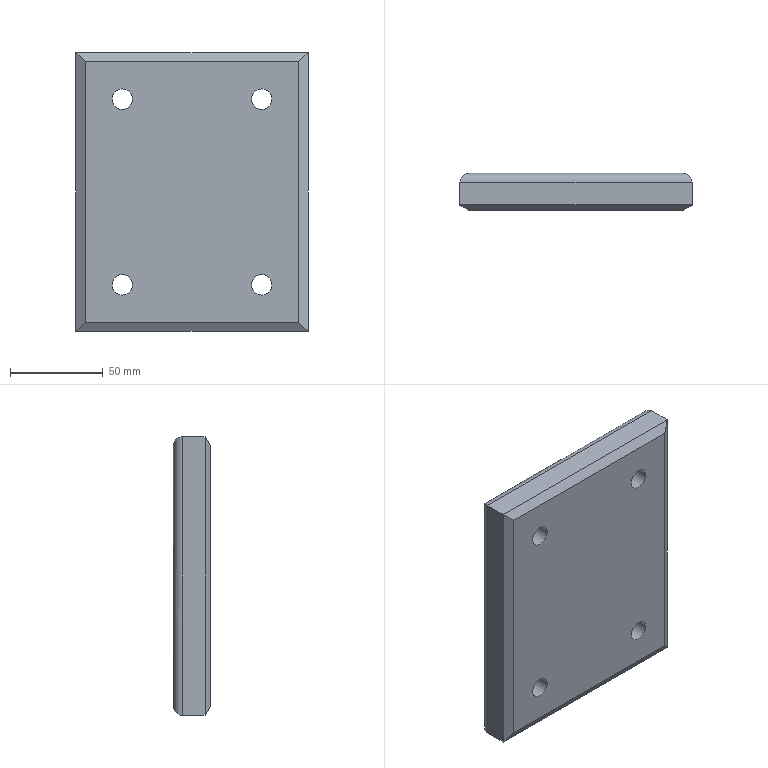Part | NX | features solid 2 | 1 solid | 30 faces | box 125 x 20 x 150 mm | volume 353028 mm3 | plane 14 | cylinder 12 | torus 4 | commonest cylinder face diameters 10 x4 11 x4 17.5 x4
STEP:
#1=CARTESIAN_POINT('',(525.,95.,-285.));
#2=VERTEX_POINT('',#1);
#3=CARTESIAN_POINT('',(640.,95.,-285.));
#4=VERTEX_POINT('',#3);
#5=CARTESIAN_POINT('',(495.,95.,-285.));
#6=DIRECTION('',(1.,0.,0.));
#7=VECTOR('',#6,1000.);
#8=LINE('',#5,#7);
#9=EDGE_CURVE('',#2,#4,#8,.T.);
#10=ORIENTED_EDGE('',*,*,#9,.F.);
#11=CARTESIAN_POINT('',(525.,95.,-145.));
#12=VERTEX_POINT('',#11);
#13=CARTESIAN_POINT('',(525.,95.,-290.));
#14=DIRECTION('',(0.,0.,-1.));
#15=VECTOR('',#14,1000.);
#16=LINE('',#13,#15);
#17=EDGE_CURVE('',#12,#2,#16,.T.);
#18=ORIENTED_EDGE('',*,*,#17,.F.);
#19=CARTESIAN_POINT('',(640.,95.,-145.));
#20=VERTEX_POINT('',#19);
#21=CARTESIAN_POINT('',(495.,95.,-145.));
#22=DIRECTION('',(-1.,0.,0.));
#23=VECTOR('',#22,1000.);
#24=LINE('',#21,#23);
#25=EDGE_CURVE('',#20,#12,#24,.T.);
#26=ORIENTED_EDGE('',*,*,#25,.F.);
#27=CARTESIAN_POINT('',(640.,95.,-290.));
#28=DIRECTION('',(0.,0.,1.));
#29=VECTOR('',#28,1000.);
#30=LINE('',#27,#29);
#31=EDGE_CURVE('',#4,#20,#30,.T.);
#32=ORIENTED_EDGE('',*,*,#31,.F.);
#33=EDGE_LOOP('',(#10,#18,#26,#32));
#34=FACE_BOUND('',#33,.T.);
#35=CARTESIAN_POINT('',(545.,95.,-253.25));
#36=VERTEX_POINT('',#35);
#37=CARTESIAN_POINT('',(545.,95.,-265.));
#38=DIRECTION('',(0.,1.,0.));
#39=DIRECTION('',(0.,0.,1.));
#40=AXIS2_PLACEMENT_3D('',#37,#38,#39);
#41=CIRCLE('',#40,11.75);
#42=EDGE_CURVE('',#36,#36,#41,.T.);
#43=ORIENTED_EDGE('',*,*,#42,.F.);
#44=EDGE_LOOP('',(#43));
#45=FACE_BOUND('',#44,.T.);
#46=CARTESIAN_POINT('',(620.,95.,-253.25));
#47=VERTEX_POINT('',#46);
#48=CARTESIAN_POINT('',(620.,95.,-265.));
#49=DIRECTION('',(0.,1.,0.));
#50=DIRECTION('',(0.,0.,1.));
#51=AXIS2_PLACEMENT_3D('',#48,#49,#50);
#52=CIRCLE('',#51,11.75);
#53=EDGE_CURVE('',#47,#47,#52,.T.);
#54=ORIENTED_EDGE('',*,*,#53,.F.);
#55=EDGE_LOOP('',(#54));
#56=FACE_BOUND('',#55,.T.);
#57=CARTESIAN_POINT('',(620.,95.,-153.25));
#58=VERTEX_POINT('',#57);
#59=CARTESIAN_POINT('',(620.,95.,-165.));
#60=DIRECTION('',(0.,1.,0.));
#61=DIRECTION('',(0.,0.,1.));
#62=AXIS2_PLACEMENT_3D('',#59,#60,#61);
#63=CIRCLE('',#62,11.75);
#64=EDGE_CURVE('',#58,#58,#63,.T.);
#65=ORIENTED_EDGE('',*,*,#64,.F.);
#66=EDGE_LOOP('',(#65));
#67=FACE_BOUND('',#66,.T.);
#68=CARTESIAN_POINT('',(545.,95.,-153.25));
#69=VERTEX_POINT('',#68);
#70=CARTESIAN_POINT('',(545.,95.,-165.));
#71=DIRECTION('',(0.,1.,0.));
#72=DIRECTION('',(0.,0.,1.));
#73=AXIS2_PLACEMENT_3D('',#70,#71,#72);
#74=CIRCLE('',#73,11.75);
#75=EDGE_CURVE('',#69,#69,#74,.T.);
#76=ORIENTED_EDGE('',*,*,#75,.F.);
#77=EDGE_LOOP('',(#76));
#78=FACE_BOUND('',#77,.T.);
#79=CARTESIAN_POINT('',(495.,95.,-290.));
#80=DIRECTION('',(0.,1.,0.));
#81=DIRECTION('',(0.,0.,-1.));
#82=AXIS2_PLACEMENT_3D('',#79,#80,#81);
#83=PLANE('',#82);
#84=ADVANCED_FACE('',(#34,#45,#56,#67,#78),#83,.T.);
#85=CARTESIAN_POINT('',(645.,90.,-140.));
#86=VERTEX_POINT('',#85);
#87=CARTESIAN_POINT('',(645.,78.,-140.));
#88=VERTEX_POINT('',#87);
#89=CARTESIAN_POINT('',(645.,95.,-140.));
#90=DIRECTION('',(0.,-1.,0.));
#91=VECTOR('',#90,1000.);
#92=LINE('',#89,#91);
#93=EDGE_CURVE('',#86,#88,#92,.T.);
#94=ORIENTED_EDGE('',*,*,#93,.F.);
#95=CARTESIAN_POINT('',(520.,90.,-140.));
#96=VERTEX_POINT('',#95);
#97=CARTESIAN_POINT('',(495.,90.,-140.));
#98=DIRECTION('',(1.,0.,0.));
#99=VECTOR('',#98,1000.);
#100=LINE('',#97,#99);
#101=EDGE_CURVE('',#96,#86,#100,.T.);
#102=ORIENTED_EDGE('',*,*,#101,.F.);
#103=CARTESIAN_POINT('',(520.,78.,-140.));
#104=VERTEX_POINT('',#103);
#105=CARTESIAN_POINT('',(520.,95.,-140.));
#106=DIRECTION('',(0.,-1.,0.));
#107=VECTOR('',#106,1000.);
#108=LINE('',#105,#107);
#109=EDGE_CURVE('',#96,#104,#108,.T.);
#110=ORIENTED_EDGE('',*,*,#109,.T.);
#111=CARTESIAN_POINT('',(495.,78.,-140.));
#112=DIRECTION('',(-1.,0.,0.));
#113=VECTOR('',#112,1000.);
#114=LINE('',#111,#113);
#115=EDGE_CURVE('',#88,#104,#114,.T.);
#116=ORIENTED_EDGE('',*,*,#115,.F.);
#117=EDGE_LOOP('',(#94,#102,#110,#116));
#118=FACE_BOUND('',#117,.T.);
#119=CARTESIAN_POINT('',(495.,95.,-140.));
#120=DIRECTION('',(0.,0.,1.));
#121=DIRECTION('',(0.,1.,0.));
#122=AXIS2_PLACEMENT_3D('',#119,#120,#121);
#123=PLANE('',#122);
#124=ADVANCED_FACE('',(#118),#123,.T.);
#125=CARTESIAN_POINT('',(640.,75.,-145.));
#126=VERTEX_POINT('',#125);
#127=CARTESIAN_POINT('',(640.,75.,-285.));
#128=VERTEX_POINT('',#127);
#129=CARTESIAN_POINT('',(640.,75.,-290.));
#130=DIRECTION('',(0.,0.,-1.));
#131=VECTOR('',#130,1000.);
#132=LINE('',#129,#131);
#133=EDGE_CURVE('',#126,#128,#132,.T.);
#134=ORIENTED_EDGE('',*,*,#133,.F.);
#135=CARTESIAN_POINT('',(525.,75.,-145.));
#136=VERTEX_POINT('',#135);
#137=CARTESIAN_POINT('',(495.,75.,-145.));
#138=DIRECTION('',(1.,0.,0.));
#139=VECTOR('',#138,1000.);
#140=LINE('',#137,#139);
#141=EDGE_CURVE('',#136,#126,#140,.T.);
#142=ORIENTED_EDGE('',*,*,#141,.F.);
#143=CARTESIAN_POINT('',(525.,75.,-285.));
#144=VERTEX_POINT('',#143);
#145=CARTESIAN_POINT('',(525.,75.,-140.));
#146=DIRECTION('',(0.,0.,1.));
#147=VECTOR('',#146,1000.);
#148=LINE('',#145,#147);
#149=EDGE_CURVE('',#144,#136,#148,.T.);
#150=ORIENTED_EDGE('',*,*,#149,.F.);
#151=CARTESIAN_POINT('',(495.,75.,-285.));
#152=DIRECTION('',(-1.,0.,0.));
#153=VECTOR('',#152,1000.);
#154=LINE('',#151,#153);
#155=EDGE_CURVE('',#128,#144,#154,.T.);
#156=ORIENTED_EDGE('',*,*,#155,.F.);
#157=EDGE_LOOP('',(#134,#142,#150,#156));
#158=FACE_BOUND('',#157,.T.);
#159=CARTESIAN_POINT('',(620.,75.,-259.5));
#160=VERTEX_POINT('',#159);
#161=CARTESIAN_POINT('',(620.,75.,-265.));
#162=DIRECTION('',(0.,1.,0.));
#163=DIRECTION('',(0.,0.,1.));
#164=AXIS2_PLACEMENT_3D('',#161,#162,#163);
#165=CIRCLE('',#164,5.5);
#166=EDGE_CURVE('',#160,#160,#165,.T.);
#167=ORIENTED_EDGE('',*,*,#166,.T.);
#168=EDGE_LOOP('',(#167));
#169=FACE_BOUND('',#168,.T.);
#170=CARTESIAN_POINT('',(545.,75.,-259.5));
#171=VERTEX_POINT('',#170);
#172=CARTESIAN_POINT('',(545.,75.,-265.));
#173=DIRECTION('',(0.,1.,0.));
#174=DIRECTION('',(0.,0.,1.));
#175=AXIS2_PLACEMENT_3D('',#172,#173,#174);
#176=CIRCLE('',#175,5.5);
#177=EDGE_CURVE('',#171,#171,#176,.T.);
#178=ORIENTED_EDGE('',*,*,#177,.T.);
#179=EDGE_LOOP('',(#178));
#180=FACE_BOUND('',#179,.T.);
#181=CARTESIAN_POINT('',(620.,75.,-159.5));
#182=VERTEX_POINT('',#181);
#183=CARTESIAN_POINT('',(620.,75.,-165.));
#184=DIRECTION('',(0.,1.,0.));
#185=DIRECTION('',(0.,0.,1.));
#186=AXIS2_PLACEMENT_3D('',#183,#184,#185);
#187=CIRCLE('',#186,5.5);
#188=EDGE_CURVE('',#182,#182,#187,.T.);
#189=ORIENTED_EDGE('',*,*,#188,.T.);
#190=EDGE_LOOP('',(#189));
#191=FACE_BOUND('',#190,.T.);
#192=CARTESIAN_POINT('',(545.,75.,-159.5));
#193=VERTEX_POINT('',#192);
#194=CARTESIAN_POINT('',(545.,75.,-165.));
#195=DIRECTION('',(0.,1.,0.));
#196=DIRECTION('',(0.,0.,1.));
#197=AXIS2_PLACEMENT_3D('',#194,#195,#196);
#198=CIRCLE('',#197,5.5);
#199=EDGE_CURVE('',#193,#193,#198,.T.);
#200=ORIENTED_EDGE('',*,*,#199,.T.);
#201=EDGE_LOOP('',(#200));
#202=FACE_BOUND('',#201,.T.);
#203=CARTESIAN_POINT('',(495.,75.,-290.));
#204=DIRECTION('',(0.,1.,0.));
#205=DIRECTION('',(0.,0.,-1.));
#206=AXIS2_PLACEMENT_3D('',#203,#204,#205);
#207=PLANE('',#206);
#208=ADVANCED_FACE('',(#158,#169,#180,#191,#202),#207,.F.);
#209=CARTESIAN_POINT('',(520.,90.,-290.));
#210=VERTEX_POINT('',#209);
#211=CARTESIAN_POINT('',(520.,78.,-290.));
#212=VERTEX_POINT('',#211);
#213=CARTESIAN_POINT('',(520.,95.,-290.));
#214=DIRECTION('',(0.,-1.,0.));
#215=VECTOR('',#214,1000.);
#216=LINE('',#213,#215);
#217=EDGE_CURVE('',#210,#212,#216,.T.);
#218=ORIENTED_EDGE('',*,*,#217,.F.);
#219=CARTESIAN_POINT('',(645.,90.,-290.));
#220=VERTEX_POINT('',#219);
#221=CARTESIAN_POINT('',(495.,90.,-290.));
#222=DIRECTION('',(-1.,0.,0.));
#223=VECTOR('',#222,1000.);
#224=LINE('',#221,#223);
#225=EDGE_CURVE('',#220,#210,#224,.T.);
#226=ORIENTED_EDGE('',*,*,#225,.F.);
#227=CARTESIAN_POINT('',(645.,78.,-290.));
#228=VERTEX_POINT('',#227);
#229=CARTESIAN_POINT('',(645.,95.,-290.));
#230=DIRECTION('',(0.,-1.,0.));
#231=VECTOR('',#230,1000.);
#232=LINE('',#229,#231);
#233=EDGE_CURVE('',#220,#228,#232,.T.);
#234=ORIENTED_EDGE('',*,*,#233,.T.);
#235=CARTESIAN_POINT('',(495.,78.,-290.));
#236=DIRECTION('',(1.,0.,0.));
#237=VECTOR('',#236,1000.);
#238=LINE('',#235,#237);
#239=EDGE_CURVE('',#212,#228,#238,.T.);
#240=ORIENTED_EDGE('',*,*,#239,.F.);
#241=EDGE_LOOP('',(#218,#226,#234,#240));
#242=FACE_BOUND('',#241,.T.);
#243=CARTESIAN_POINT('',(495.,95.,-290.));
#244=DIRECTION('',(0.,0.,1.));
#245=DIRECTION('',(0.,1.,0.));
#246=AXIS2_PLACEMENT_3D('',#243,#244,#245);
#247=PLANE('',#246);
#248=ADVANCED_FACE('',(#242),#247,.F.);
#249=ORIENTED_EDGE('',*,*,#233,.F.);
#250=CARTESIAN_POINT('',(645.,90.,-290.));
#251=DIRECTION('',(0.,0.,-1.));
#252=VECTOR('',#251,1000.);
#253=LINE('',#250,#252);
#254=EDGE_CURVE('',#86,#220,#253,.T.);
#255=ORIENTED_EDGE('',*,*,#254,.F.);
#256=ORIENTED_EDGE('',*,*,#93,.T.);
#257=CARTESIAN_POINT('',(645.,78.,-290.));
#258=DIRECTION('',(0.,0.,1.));
#259=VECTOR('',#258,1000.);
#260=LINE('',#257,#259);
#261=EDGE_CURVE('',#228,#88,#260,.T.);
#262=ORIENTED_EDGE('',*,*,#261,.F.);
#263=EDGE_LOOP('',(#249,#255,#256,#262));
#264=FACE_BOUND('',#263,.T.);
#265=CARTESIAN_POINT('',(645.,95.,-290.));
#266=DIRECTION('',(1.,0.,0.));
#267=DIRECTION('',(0.,0.,-1.));
#268=AXIS2_PLACEMENT_3D('',#265,#266,#267);
#269=PLANE('',#268);
#270=ADVANCED_FACE('',(#264),#269,.T.);
#271=ORIENTED_EDGE('',*,*,#109,.F.);
#272=CARTESIAN_POINT('',(520.,90.,-140.));
#273=DIRECTION('',(0.,0.,1.));
#274=VECTOR('',#273,1000.);
#275=LINE('',#272,#274);
#276=EDGE_CURVE('',#210,#96,#275,.T.);
#277=ORIENTED_EDGE('',*,*,#276,.F.);
#278=ORIENTED_EDGE('',*,*,#217,.T.);
#279=CARTESIAN_POINT('',(520.,78.,-290.));
#280=DIRECTION('',(0.,0.,-1.));
#281=VECTOR('',#280,1000.);
#282=LINE('',#279,#281);
#283=EDGE_CURVE('',#104,#212,#282,.T.);
#284=ORIENTED_EDGE('',*,*,#283,.F.);
#285=EDGE_LOOP('',(#271,#277,#278,#284));
#286=FACE_BOUND('',#285,.T.);
#287=CARTESIAN_POINT('',(520.,95.,-290.));
#288=DIRECTION('',(1.,0.,0.));
#289=DIRECTION('',(0.,0.,-1.));
#290=AXIS2_PLACEMENT_3D('',#287,#288,#289);
#291=PLANE('',#290);
#292=ADVANCED_FACE('',(#286),#291,.F.);
#293=ORIENTED_EDGE('',*,*,#199,.F.);
#294=EDGE_LOOP('',(#293));
#295=FACE_BOUND('',#294,.T.);
#296=CARTESIAN_POINT('',(545.,83.,-170.5));
#297=VERTEX_POINT('',#296);
#298=CARTESIAN_POINT('',(545.,83.,-165.));
#299=DIRECTION('',(0.,1.,0.));
#300=DIRECTION('',(0.,0.,-1.));
#301=AXIS2_PLACEMENT_3D('',#298,#299,#300);
#302=CIRCLE('',#301,5.5);
#303=EDGE_CURVE('',#297,#297,#302,.T.);
#304=ORIENTED_EDGE('',*,*,#303,.T.);
#305=EDGE_LOOP('',(#304));
#306=FACE_BOUND('',#305,.T.);
#307=CARTESIAN_POINT('',(545.,45.,-165.));
#308=DIRECTION('',(0.,-1.,0.));
#309=DIRECTION('',(0.,0.,1.));
#310=AXIS2_PLACEMENT_3D('',#307,#308,#309);
#311=CYLINDRICAL_SURFACE('',#310,5.5);
#312=ADVANCED_FACE('',(#295,#306),#311,.F.);
#313=ORIENTED_EDGE('',*,*,#303,.F.);
#314=EDGE_LOOP('',(#313));
#315=FACE_BOUND('',#314,.T.);
#316=CARTESIAN_POINT('',(545.,83.,-173.75));
#317=VERTEX_POINT('',#316);
#318=CARTESIAN_POINT('',(545.,83.,-165.));
#319=DIRECTION('',(0.,1.,0.));
#320=DIRECTION('',(0.,0.,-1.));
#321=AXIS2_PLACEMENT_3D('',#318,#319,#320);
#322=CIRCLE('',#321,8.75);
#323=EDGE_CURVE('',#317,#317,#322,.T.);
#324=ORIENTED_EDGE('',*,*,#323,.T.);
#325=EDGE_LOOP('',(#324));
#326=FACE_BOUND('',#325,.T.);
#327=CARTESIAN_POINT('',(545.,83.,-165.));
#328=DIRECTION('',(0.,-1.,0.));
#329=DIRECTION('',(0.,0.,1.));
#330=AXIS2_PLACEMENT_3D('',#327,#328,#329);
#331=PLANE('',#330);
#332=ADVANCED_FACE('',(#315,#326),#331,.F.);
#333=CARTESIAN_POINT('',(545.,92.,-156.25));
#334=VERTEX_POINT('',#333);
#335=CARTESIAN_POINT('',(545.,92.,-165.));
#336=DIRECTION('',(0.,-1.,0.));
#337=DIRECTION('',(0.,0.,1.));
#338=AXIS2_PLACEMENT_3D('',#335,#336,#337);
#339=CIRCLE('',#338,8.75);
#340=EDGE_CURVE('',#334,#334,#339,.T.);
#341=ORIENTED_EDGE('',*,*,#340,.F.);
#342=EDGE_LOOP('',(#341));
#343=FACE_BOUND('',#342,.T.);
#344=ORIENTED_EDGE('',*,*,#323,.F.);
#345=EDGE_LOOP('',(#344));
#346=FACE_BOUND('',#345,.T.);
#347=CARTESIAN_POINT('',(545.,95.,-165.));
#348=DIRECTION('',(0.,-1.,0.));
#349=DIRECTION('',(0.,0.,1.));
#350=AXIS2_PLACEMENT_3D('',#347,#348,#349);
#351=CYLINDRICAL_SURFACE('',#350,8.75);
#352=ADVANCED_FACE('',(#343,#346),#351,.F.);
#353=ORIENTED_EDGE('',*,*,#188,.F.);
#354=EDGE_LOOP('',(#353));
#355=FACE_BOUND('',#354,.T.);
#356=CARTESIAN_POINT('',(620.,83.,-170.5));
#357=VERTEX_POINT('',#356);
#358=CARTESIAN_POINT('',(620.,83.,-165.));
#359=DIRECTION('',(0.,1.,0.));
#360=DIRECTION('',(0.,0.,-1.));
#361=AXIS2_PLACEMENT_3D('',#358,#359,#360);
#362=CIRCLE('',#361,5.5);
#363=EDGE_CURVE('',#357,#357,#362,.T.);
#364=ORIENTED_EDGE('',*,*,#363,.T.);
#365=EDGE_LOOP('',(#364));
#366=FACE_BOUND('',#365,.T.);
#367=CARTESIAN_POINT('',(620.,45.,-165.));
#368=DIRECTION('',(0.,-1.,0.));
#369=DIRECTION('',(0.,0.,1.));
#370=AXIS2_PLACEMENT_3D('',#367,#368,#369);
#371=CYLINDRICAL_SURFACE('',#370,5.5);
#372=ADVANCED_FACE('',(#355,#366),#371,.F.);
#373=ORIENTED_EDGE('',*,*,#363,.F.);
#374=EDGE_LOOP('',(#373));
#375=FACE_BOUND('',#374,.T.);
#376=CARTESIAN_POINT('',(620.,83.,-173.75));
#377=VERTEX_POINT('',#376);
#378=CARTESIAN_POINT('',(620.,83.,-165.));
#379=DIRECTION('',(0.,1.,0.));
#380=DIRECTION('',(0.,0.,-1.));
#381=AXIS2_PLACEMENT_3D('',#378,#379,#380);
#382=CIRCLE('',#381,8.75);
#383=EDGE_CURVE('',#377,#377,#382,.T.);
#384=ORIENTED_EDGE('',*,*,#383,.T.);
#385=EDGE_LOOP('',(#384));
#386=FACE_BOUND('',#385,.T.);
#387=CARTESIAN_POINT('',(620.,83.,-165.));
#388=DIRECTION('',(0.,-1.,0.));
#389=DIRECTION('',(0.,0.,1.));
#390=AXIS2_PLACEMENT_3D('',#387,#388,#389);
#391=PLANE('',#390);
#392=ADVANCED_FACE('',(#375,#386),#391,.F.);
#393=CARTESIAN_POINT('',(620.,92.,-156.25));
#394=VERTEX_POINT('',#393);
#395=CARTESIAN_POINT('',(620.,92.,-165.));
#396=DIRECTION('',(0.,-1.,0.));
#397=DIRECTION('',(0.,0.,1.));
#398=AXIS2_PLACEMENT_3D('',#395,#396,#397);
#399=CIRCLE('',#398,8.75);
#400=EDGE_CURVE('',#394,#394,#399,.T.);
#401=ORIENTED_EDGE('',*,*,#400,.F.);
#402=EDGE_LOOP('',(#401));
#403=FACE_BOUND('',#402,.T.);
#404=ORIENTED_EDGE('',*,*,#383,.F.);
#405=EDGE_LOOP('',(#404));
#406=FACE_BOUND('',#405,.T.);
#407=CARTESIAN_POINT('',(620.,95.,-165.));
#408=DIRECTION('',(0.,-1.,0.));
#409=DIRECTION('',(0.,0.,1.));
#410=AXIS2_PLACEMENT_3D('',#407,#408,#409);
#411=CYLINDRICAL_SURFACE('',#410,8.75);
#412=ADVANCED_FACE('',(#403,#406),#411,.F.);
#413=ORIENTED_EDGE('',*,*,#177,.F.);
#414=EDGE_LOOP('',(#413));
#415=FACE_BOUND('',#414,.T.);
#416=CARTESIAN_POINT('',(545.,83.,-270.5));
#417=VERTEX_POINT('',#416);
#418=CARTESIAN_POINT('',(545.,83.,-265.));
#419=DIRECTION('',(0.,1.,0.));
#420=DIRECTION('',(0.,0.,-1.));
#421=AXIS2_PLACEMENT_3D('',#418,#419,#420);
#422=CIRCLE('',#421,5.5);
#423=EDGE_CURVE('',#417,#417,#422,.T.);
#424=ORIENTED_EDGE('',*,*,#423,.T.);
#425=EDGE_LOOP('',(#424));
#426=FACE_BOUND('',#425,.T.);
#427=CARTESIAN_POINT('',(545.,45.,-265.));
#428=DIRECTION('',(0.,-1.,0.));
#429=DIRECTION('',(0.,0.,1.));
#430=AXIS2_PLACEMENT_3D('',#427,#428,#429);
#431=CYLINDRICAL_SURFACE('',#430,5.5);
#432=ADVANCED_FACE('',(#415,#426),#431,.F.);
#433=ORIENTED_EDGE('',*,*,#423,.F.);
#434=EDGE_LOOP('',(#433));
#435=FACE_BOUND('',#434,.T.);
#436=CARTESIAN_POINT('',(545.,83.,-273.75));
#437=VERTEX_POINT('',#436);
#438=CARTESIAN_POINT('',(545.,83.,-265.));
#439=DIRECTION('',(0.,1.,0.));
#440=DIRECTION('',(0.,0.,-1.));
#441=AXIS2_PLACEMENT_3D('',#438,#439,#440);
#442=CIRCLE('',#441,8.75);
#443=EDGE_CURVE('',#437,#437,#442,.T.);
#444=ORIENTED_EDGE('',*,*,#443,.T.);
#445=EDGE_LOOP('',(#444));
#446=FACE_BOUND('',#445,.T.);
#447=CARTESIAN_POINT('',(545.,83.,-265.));
#448=DIRECTION('',(0.,-1.,0.));
#449=DIRECTION('',(0.,0.,1.));
#450=AXIS2_PLACEMENT_3D('',#447,#448,#449);
#451=PLANE('',#450);
#452=ADVANCED_FACE('',(#435,#446),#451,.F.);
#453=CARTESIAN_POINT('',(545.,92.,-256.25));
#454=VERTEX_POINT('',#453);
#455=CARTESIAN_POINT('',(545.,92.,-265.));
#456=DIRECTION('',(0.,-1.,0.));
#457=DIRECTION('',(0.,0.,1.));
#458=AXIS2_PLACEMENT_3D('',#455,#456,#457);
#459=CIRCLE('',#458,8.75);
#460=EDGE_CURVE('',#454,#454,#459,.T.);
#461=ORIENTED_EDGE('',*,*,#460,.F.);
#462=EDGE_LOOP('',(#461));
#463=FACE_BOUND('',#462,.T.);
#464=ORIENTED_EDGE('',*,*,#443,.F.);
#465=EDGE_LOOP('',(#464));
#466=FACE_BOUND('',#465,.T.);
#467=CARTESIAN_POINT('',(545.,95.,-265.));
#468=DIRECTION('',(0.,-1.,0.));
#469=DIRECTION('',(0.,0.,1.));
#470=AXIS2_PLACEMENT_3D('',#467,#468,#469);
#471=CYLINDRICAL_SURFACE('',#470,8.75);
#472=ADVANCED_FACE('',(#463,#466),#471,.F.);
#473=ORIENTED_EDGE('',*,*,#166,.F.);
#474=EDGE_LOOP('',(#473));
#475=FACE_BOUND('',#474,.T.);
#476=CARTESIAN_POINT('',(620.,83.,-270.5));
#477=VERTEX_POINT('',#476);
#478=CARTESIAN_POINT('',(620.,83.,-265.));
#479=DIRECTION('',(0.,1.,0.));
#480=DIRECTION('',(0.,0.,-1.));
#481=AXIS2_PLACEMENT_3D('',#478,#479,#480);
#482=CIRCLE('',#481,5.5);
#483=EDGE_CURVE('',#477,#477,#482,.T.);
#484=ORIENTED_EDGE('',*,*,#483,.T.);
#485=EDGE_LOOP('',(#484));
#486=FACE_BOUND('',#485,.T.);
#487=CARTESIAN_POINT('',(620.,45.,-265.));
#488=DIRECTION('',(0.,-1.,0.));
#489=DIRECTION('',(0.,0.,1.));
#490=AXIS2_PLACEMENT_3D('',#487,#488,#489);
#491=CYLINDRICAL_SURFACE('',#490,5.5);
#492=ADVANCED_FACE('',(#475,#486),#491,.F.);
#493=ORIENTED_EDGE('',*,*,#483,.F.);
#494=EDGE_LOOP('',(#493));
#495=FACE_BOUND('',#494,.T.);
#496=CARTESIAN_POINT('',(620.,83.,-273.75));
#497=VERTEX_POINT('',#496);
#498=CARTESIAN_POINT('',(620.,83.,-265.));
#499=DIRECTION('',(0.,1.,0.));
#500=DIRECTION('',(0.,0.,-1.));
#501=AXIS2_PLACEMENT_3D('',#498,#499,#500);
#502=CIRCLE('',#501,8.75);
#503=EDGE_CURVE('',#497,#497,#502,.T.);
#504=ORIENTED_EDGE('',*,*,#503,.T.);
#505=EDGE_LOOP('',(#504));
#506=FACE_BOUND('',#505,.T.);
#507=CARTESIAN_POINT('',(620.,83.,-265.));
#508=DIRECTION('',(0.,-1.,0.));
#509=DIRECTION('',(0.,0.,1.));
#510=AXIS2_PLACEMENT_3D('',#507,#508,#509);
#511=PLANE('',#510);
#512=ADVANCED_FACE('',(#495,#506),#511,.F.);
#513=CARTESIAN_POINT('',(620.,92.,-256.25));
#514=VERTEX_POINT('',#513);
#515=CARTESIAN_POINT('',(620.,92.,-265.));
#516=DIRECTION('',(0.,-1.,0.));
#517=DIRECTION('',(0.,0.,1.));
#518=AXIS2_PLACEMENT_3D('',#515,#516,#517);
#519=CIRCLE('',#518,8.75);
#520=EDGE_CURVE('',#514,#514,#519,.T.);
#521=ORIENTED_EDGE('',*,*,#520,.F.);
#522=EDGE_LOOP('',(#521));
#523=FACE_BOUND('',#522,.T.);
#524=ORIENTED_EDGE('',*,*,#503,.F.);
#525=EDGE_LOOP('',(#524));
#526=FACE_BOUND('',#525,.T.);
#527=CARTESIAN_POINT('',(620.,95.,-265.));
#528=DIRECTION('',(0.,-1.,0.));
#529=DIRECTION('',(0.,0.,1.));
#530=AXIS2_PLACEMENT_3D('',#527,#528,#529);
#531=CYLINDRICAL_SURFACE('',#530,8.75);
#532=ADVANCED_FACE('',(#523,#526),#531,.F.);
#533=ORIENTED_EDGE('',*,*,#460,.T.);
#534=EDGE_LOOP('',(#533));
#535=FACE_BOUND('',#534,.T.);
#536=ORIENTED_EDGE('',*,*,#42,.T.);
#537=EDGE_LOOP('',(#536));
#538=FACE_BOUND('',#537,.T.);
#539=CARTESIAN_POINT('',(545.,92.,-265.));
#540=DIRECTION('',(0.,1.,0.));
#541=DIRECTION('',(0.,0.,-1.));
#542=AXIS2_PLACEMENT_3D('',#539,#540,#541);
#543=TOROIDAL_SURFACE('',#542,11.75,3.);
#544=ADVANCED_FACE('',(#535,#538),#543,.T.);
#545=ORIENTED_EDGE('',*,*,#520,.T.);
#546=EDGE_LOOP('',(#545));
#547=FACE_BOUND('',#546,.T.);
#548=ORIENTED_EDGE('',*,*,#53,.T.);
#549=EDGE_LOOP('',(#548));
#550=FACE_BOUND('',#549,.T.);
#551=CARTESIAN_POINT('',(620.,92.,-265.));
#552=DIRECTION('',(0.,1.,0.));
#553=DIRECTION('',(0.,0.,-1.));
#554=AXIS2_PLACEMENT_3D('',#551,#552,#553);
#555=TOROIDAL_SURFACE('',#554,11.75,3.);
#556=ADVANCED_FACE('',(#547,#550),#555,.T.);
#557=ORIENTED_EDGE('',*,*,#400,.T.);
#558=EDGE_LOOP('',(#557));
#559=FACE_BOUND('',#558,.T.);
#560=ORIENTED_EDGE('',*,*,#64,.T.);
#561=EDGE_LOOP('',(#560));
#562=FACE_BOUND('',#561,.T.);
#563=CARTESIAN_POINT('',(620.,92.,-165.));
#564=DIRECTION('',(0.,1.,0.));
#565=DIRECTION('',(0.,0.,-1.));
#566=AXIS2_PLACEMENT_3D('',#563,#564,#565);
#567=TOROIDAL_SURFACE('',#566,11.75,3.);
#568=ADVANCED_FACE('',(#559,#562),#567,.T.);
#569=ORIENTED_EDGE('',*,*,#340,.T.);
#570=EDGE_LOOP('',(#569));
#571=FACE_BOUND('',#570,.T.);
#572=ORIENTED_EDGE('',*,*,#75,.T.);
#573=EDGE_LOOP('',(#572));
#574=FACE_BOUND('',#573,.T.);
#575=CARTESIAN_POINT('',(545.,92.,-165.));
#576=DIRECTION('',(0.,1.,0.));
#577=DIRECTION('',(0.,0.,-1.));
#578=AXIS2_PLACEMENT_3D('',#575,#576,#577);
#579=TOROIDAL_SURFACE('',#578,11.75,3.);
#580=ADVANCED_FACE('',(#571,#574),#579,.T.);
#581=CARTESIAN_POINT('',(525.,90.,-145.));
#582=DIRECTION('',(-0.7071,0.,-0.7071));
#583=DIRECTION('',(0.7071,0.,-0.7071));
#584=AXIS2_PLACEMENT_3D('',#581,#582,#583);
#585=ELLIPSE('',#584,7.071,5.);
#586=EDGE_CURVE('',#96,#12,#585,.T.);
#587=ORIENTED_EDGE('',*,*,#586,.T.);
#588=ORIENTED_EDGE('',*,*,#17,.T.);
#589=CARTESIAN_POINT('',(525.,90.,-285.));
#590=DIRECTION('',(-0.7071,0.,0.7071));
#591=DIRECTION('',(-0.7071,0.,-0.7071));
#592=AXIS2_PLACEMENT_3D('',#589,#590,#591);
#593=ELLIPSE('',#592,7.071,5.);
#594=EDGE_CURVE('',#2,#210,#593,.T.);
#595=ORIENTED_EDGE('',*,*,#594,.T.);
#596=ORIENTED_EDGE('',*,*,#276,.T.);
#597=EDGE_LOOP('',(#587,#588,#595,#596));
#598=FACE_BOUND('',#597,.T.);
#599=CARTESIAN_POINT('',(525.,90.,-290.));
#600=DIRECTION('',(0.,0.,-1.));
#601=DIRECTION('',(-1.,0.,0.));
#602=AXIS2_PLACEMENT_3D('',#599,#600,#601);
#603=CYLINDRICAL_SURFACE('',#602,5.);
#604=ADVANCED_FACE('',(#598),#603,.T.);
#605=ORIENTED_EDGE('',*,*,#594,.F.);
#606=ORIENTED_EDGE('',*,*,#9,.T.);
#607=CARTESIAN_POINT('',(640.,90.,-285.));
#608=DIRECTION('',(-0.7071,0.,-0.7071));
#609=DIRECTION('',(-0.7071,0.,0.7071));
#610=AXIS2_PLACEMENT_3D('',#607,#608,#609);
#611=ELLIPSE('',#610,7.071,5.);
#612=EDGE_CURVE('',#4,#220,#611,.T.);
#613=ORIENTED_EDGE('',*,*,#612,.T.);
#614=ORIENTED_EDGE('',*,*,#225,.T.);
#615=EDGE_LOOP('',(#605,#606,#613,#614));
#616=FACE_BOUND('',#615,.T.);
#617=CARTESIAN_POINT('',(495.,90.,-285.));
#618=DIRECTION('',(-1.,0.,0.));
#619=DIRECTION('',(0.,0.,1.));
#620=AXIS2_PLACEMENT_3D('',#617,#618,#619);
#621=CYLINDRICAL_SURFACE('',#620,5.);
#622=ADVANCED_FACE('',(#616),#621,.T.);
#623=ORIENTED_EDGE('',*,*,#586,.F.);
#624=ORIENTED_EDGE('',*,*,#101,.T.);
#625=CARTESIAN_POINT('',(640.,90.,-145.));
#626=DIRECTION('',(-0.7071,0.,0.7071));
#627=DIRECTION('',(0.7071,0.,0.7071));
#628=AXIS2_PLACEMENT_3D('',#625,#626,#627);
#629=ELLIPSE('',#628,7.071,5.);
#630=EDGE_CURVE('',#86,#20,#629,.T.);
#631=ORIENTED_EDGE('',*,*,#630,.T.);
#632=ORIENTED_EDGE('',*,*,#25,.T.);
#633=EDGE_LOOP('',(#623,#624,#631,#632));
#634=FACE_BOUND('',#633,.T.);
#635=CARTESIAN_POINT('',(495.,90.,-145.));
#636=DIRECTION('',(1.,0.,0.));
#637=DIRECTION('',(0.,0.,-1.));
#638=AXIS2_PLACEMENT_3D('',#635,#636,#637);
#639=CYLINDRICAL_SURFACE('',#638,5.);
#640=ADVANCED_FACE('',(#634),#639,.T.);
#641=ORIENTED_EDGE('',*,*,#612,.F.);
#642=ORIENTED_EDGE('',*,*,#31,.T.);
#643=ORIENTED_EDGE('',*,*,#630,.F.);
#644=ORIENTED_EDGE('',*,*,#254,.T.);
#645=EDGE_LOOP('',(#641,#642,#643,#644));
#646=FACE_BOUND('',#645,.T.);
#647=CARTESIAN_POINT('',(640.,90.,-290.));
#648=DIRECTION('',(0.,0.,1.));
#649=DIRECTION('',(1.,0.,0.));
#650=AXIS2_PLACEMENT_3D('',#647,#648,#649);
#651=CYLINDRICAL_SURFACE('',#650,5.);
#652=ADVANCED_FACE('',(#646),#651,.T.);
#653=CARTESIAN_POINT('',(581.441,39.864,-203.559));
#654=DIRECTION('',(0.6509,0.3906,0.6509));
#655=VECTOR('',#654,1000.);
#656=LINE('',#653,#655);
#657=EDGE_CURVE('',#126,#88,#656,.T.);
#658=ORIENTED_EDGE('',*,*,#657,.T.);
#659=ORIENTED_EDGE('',*,*,#115,.T.);
#660=CARTESIAN_POINT('',(512.288,82.627,-132.288));
#661=DIRECTION('',(0.6509,-0.3906,-0.6509));
#662=VECTOR('',#661,1000.);
#663=LINE('',#660,#662);
#664=EDGE_CURVE('',#104,#136,#663,.T.);
#665=ORIENTED_EDGE('',*,*,#664,.T.);
#666=ORIENTED_EDGE('',*,*,#141,.T.);
#667=EDGE_LOOP('',(#658,#659,#665,#666));
#668=FACE_BOUND('',#667,.T.);
#669=CARTESIAN_POINT('',(495.,75.,-145.));
#670=DIRECTION('',(0.,-0.8575,0.5145));
#671=DIRECTION('',(0.,0.5145,0.8575));
#672=AXIS2_PLACEMENT_3D('',#669,#670,#671);
#673=PLANE('',#672);
#674=ADVANCED_FACE('',(#668),#673,.T.);
#675=ORIENTED_EDGE('',*,*,#664,.F.);
#676=ORIENTED_EDGE('',*,*,#283,.T.);
#677=CARTESIAN_POINT('',(522.881,76.271,-287.119));
#678=DIRECTION('',(0.6509,-0.3906,0.6509));
#679=VECTOR('',#678,1000.);
#680=LINE('',#677,#679);
#681=EDGE_CURVE('',#212,#144,#680,.T.);
#682=ORIENTED_EDGE('',*,*,#681,.T.);
#683=ORIENTED_EDGE('',*,*,#149,.T.);
#684=EDGE_LOOP('',(#675,#676,#682,#683));
#685=FACE_BOUND('',#684,.T.);
#686=CARTESIAN_POINT('',(525.,75.,-290.));
#687=DIRECTION('',(0.5145,0.8575,0.));
#688=DIRECTION('',(-0.8575,0.5145,0.));
#689=AXIS2_PLACEMENT_3D('',#686,#687,#688);
#690=PLANE('',#689);
#691=ADVANCED_FACE('',(#685),#690,.F.);
#692=ORIENTED_EDGE('',*,*,#657,.F.);
#693=ORIENTED_EDGE('',*,*,#133,.T.);
#694=CARTESIAN_POINT('',(645.,78.,-290.));
#695=DIRECTION('',(0.6509,0.3906,-0.6509));
#696=VECTOR('',#695,1000.);
#697=LINE('',#694,#696);
#698=EDGE_CURVE('',#128,#228,#697,.T.);
#699=ORIENTED_EDGE('',*,*,#698,.T.);
#700=ORIENTED_EDGE('',*,*,#261,.T.);
#701=EDGE_LOOP('',(#692,#693,#699,#700));
#702=FACE_BOUND('',#701,.T.);
#703=CARTESIAN_POINT('',(645.,78.,-290.));
#704=DIRECTION('',(0.5145,-0.8575,0.));
#705=DIRECTION('',(0.8575,0.5145,0.));
#706=AXIS2_PLACEMENT_3D('',#703,#704,#705);
#707=PLANE('',#706);
#708=ADVANCED_FACE('',(#702),#707,.T.);
#709=ORIENTED_EDGE('',*,*,#681,.F.);
#710=ORIENTED_EDGE('',*,*,#239,.T.);
#711=ORIENTED_EDGE('',*,*,#698,.F.);
#712=ORIENTED_EDGE('',*,*,#155,.T.);
#713=EDGE_LOOP('',(#709,#710,#711,#712));
#714=FACE_BOUND('',#713,.T.);
#715=CARTESIAN_POINT('',(495.,78.,-290.));
#716=DIRECTION('',(0.,0.8575,0.5145));
#717=DIRECTION('',(0.,0.5145,-0.8575));
#718=AXIS2_PLACEMENT_3D('',#715,#716,#717);
#719=PLANE('',#718);
#720=ADVANCED_FACE('',(#714),#719,.F.);
#721=CLOSED_SHELL('',(#84,#124,#208,#248,#270,#292,#312,#332,#352,#372,#392,#412,#432,#452,#472,#492,#512,#532,#544,#556,#568,#580,#604,#622,#640,#652,#674,#691,#708,#720));
#722=MANIFOLD_SOLID_BREP('',#721);
#723=(LENGTH_UNIT()NAMED_UNIT(*)SI_UNIT(.MILLI.,.METRE.));
#724=UNCERTAINTY_MEASURE_WITH_UNIT(LENGTH_MEASURE(0.00001),#723,'','');
#725=(NAMED_UNIT(*)PLANE_ANGLE_UNIT()SI_UNIT($,.RADIAN.));
#726=(NAMED_UNIT(*)SI_UNIT($,.STERADIAN.)SOLID_ANGLE_UNIT());
#727=(GEOMETRIC_REPRESENTATION_CONTEXT(3)GLOBAL_UNCERTAINTY_ASSIGNED_CONTEXT((#724))GLOBAL_UNIT_ASSIGNED_CONTEXT((#723,#725,#726))REPRESENTATION_CONTEXT('',''));
#728=ADVANCED_BREP_SHAPE_REPRESENTATION('',(#722),#727);